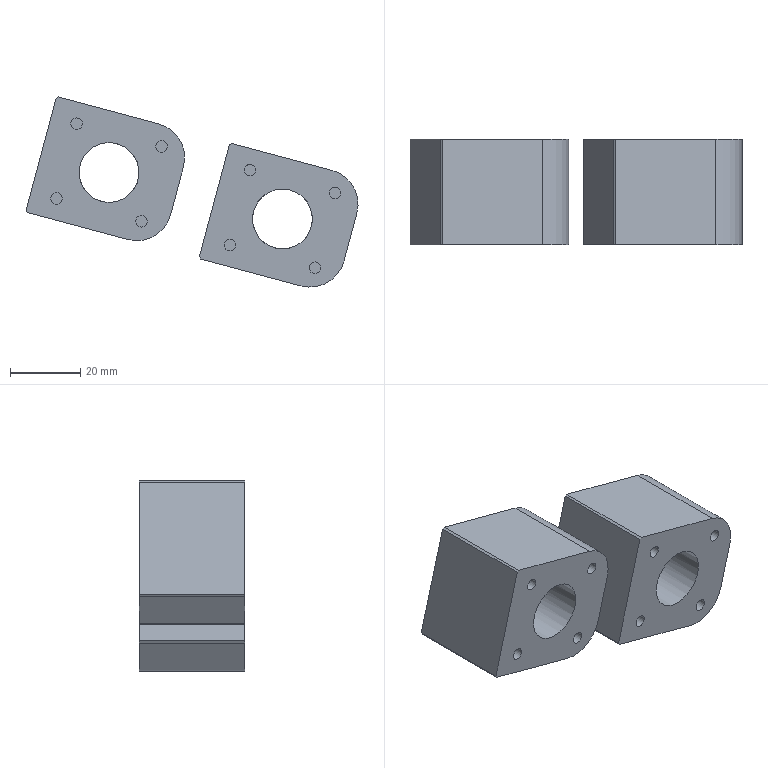CAM job | NX | 3+2 milling, drilling | part box 94.322 x 30 x 54.017 mm | stock box 101.788 x 35 x 58.654 mm
Tools:
number,name,description,diameter,corner_radius,flute_length,length,flutes
9,D10,平底铣刀-粗,10.0,0.0,35.0,75.0,2
10,D10-J,平底铣刀-精,10.0,0.0,35.0,75.0,2
1,D80R0.8飞刀,圆鼻刀-粗,80.0,0.8,50.0,75.0,2
1,D80R0.8飞刀-J,圆鼻刀-精,80.0,0.8,50.0,75.0,2
2,D6倒角刀,倒角刀,6.0,0.0,3.0,25.0,2
21,M4X0.7,丝锥,3.3,0.0,35.0,50.0,2
17,ZT12,钻头,12.0,0.0,35.0,50.0,2
13,钻头3.3,Twist Drill 3.3 mm,3.3,0.0,35.0,35.008,2
Operations:
program,operation,operation_type,tool,method,geometry_group,spindle_rpm,surface_speed,feed_per_tooth,feed_cut,feed_plunge,cut_length_mm,path_length_mm,cut_time_min,machine_time_min
B,底壁铣飞面一刀开粗_COPY,VolumeBased25DMillingOperation,D80R0.8飞刀,分层开粗-切深K-步距G,W-B,2800.0,703.696,0.5357,3000.0,100.0,1793.042,3553.526,0.5977,0.7737
B,底壁铣飞面一刀精光_COPY,VolumeBased25DMillingOperation,D80R0.8飞刀-J,侧刃精光-切深K-步距G,W-B,4000.0,1005.28,0.125,1000.0,100.0,199.031,235.031,0.199,0.2026
B,打点-深0.8,Operation,D6倒角刀,NONE,W-B,8000.0,150.796,0.0312,500.0,90.0,18.0,265.833,0.036,0.0608
B,盲平孔-M4螺纹底孔,Operation,钻头3.3,NONE,W-B,3000.0,31.102,0.0167,100.0,90.0,136.0,483.15,1.36,1.395
B,钻倒角_1,Operation,D6倒角刀,METHOD,W-B,8000.0,150.796,0.0312,500.0,0.0,41.6,309.546,0.0832,0.11
B,铣倒角_1,PlanarMilling,D6倒角刀,METHOD,W-B,8000.0,150.796,0.0625,1000.0,100.0,115.097,255.914,0.1151,0.1292
B,盲平孔-攻牙M4,Operation,M4X0.7,METHOD,W-B,800.0,8.294,0.0004,0.7,90.0,112.0,435.15,160.0,160.032
B,C0.3封闭铣廓倒角6X45L_COPY,PlanarMilling,D6倒角刀,爬面_倒角-切深0-步距G,W-B,7000.0,131.0,0.1071,1500.0,100.0,319.445,449.335,0.213,0.226
A,顶面,FaceMilling,D80R0.8飞刀,侧刃精光-切深K-步距G,W-A,4000.0,1005.31,0.125,1000.0,100.0,185.0,221.0,0.185,0.1886
A,外形粗_2,VolumeBased25DMillingOperation,D10,METHOD,W-A,8000.0,251.327,0.3125,5000.0,80.0,13673.093,13885.865,2.735,2.756
A,沉头孔打点-深0.8,Operation,D6倒角刀,NONE,W-A,8000.0,150.796,0.0312,500.0,90.0,3.6,99.21,0.0072,0.0168
A,沉头孔-钻孔0段,Operation,ZT12,NONE,W-A,1200.0,64.088,0.0625,150.0,90.0,78.0,248.01,0.52,0.537
A,底壁铣螺旋开粗-中_COPY,VolumeBased25DMillingOperation,D10,分层开粗-切深K-步距G,W-A,8000.0,251.327,0.1875,3000.0,100.0,1722.456,1871.25,0.5742,0.589
A,底壁铣螺旋开粗-中_COPY_COPY,VolumeBased25DMillingOperation,D10,分层开粗-切深K-步距G,W-A,8000.0,251.327,0.125,2000.0,100.0,2049.654,2249.924,1.025,1.045
A,底壁铣精光侧面-中_COPY,VolumeBased25DMillingOperation,D10-J,侧刃精光-切深K-步距G,W-A,8000.0,251.32,0.0625,1000.0,100.0,191.147,401.055,0.1911,0.2121
A,仅选体,SurfaceContour,D6倒角刀,METHOD,W-A,8000.0,150.796,0.1875,3000.0,100.0,606.731,1025.306,0.2022,0.2441
A,底壁铣精光侧面-中-选底面_COPY,VolumeBased25DMillingOperation,D10-J,侧刃精光-切深K-步距G,W-A,8000.0,251.327,0.0625,1000.0,100.0,150.656,268.77,0.1507,0.1625
A,外形半精_2,VolumeBased25DMillingOperation,D10-J,METHOD,W-A,8000.0,251.327,0.0625,1000.0,100.0,700.984,1201.023,0.701,0.751